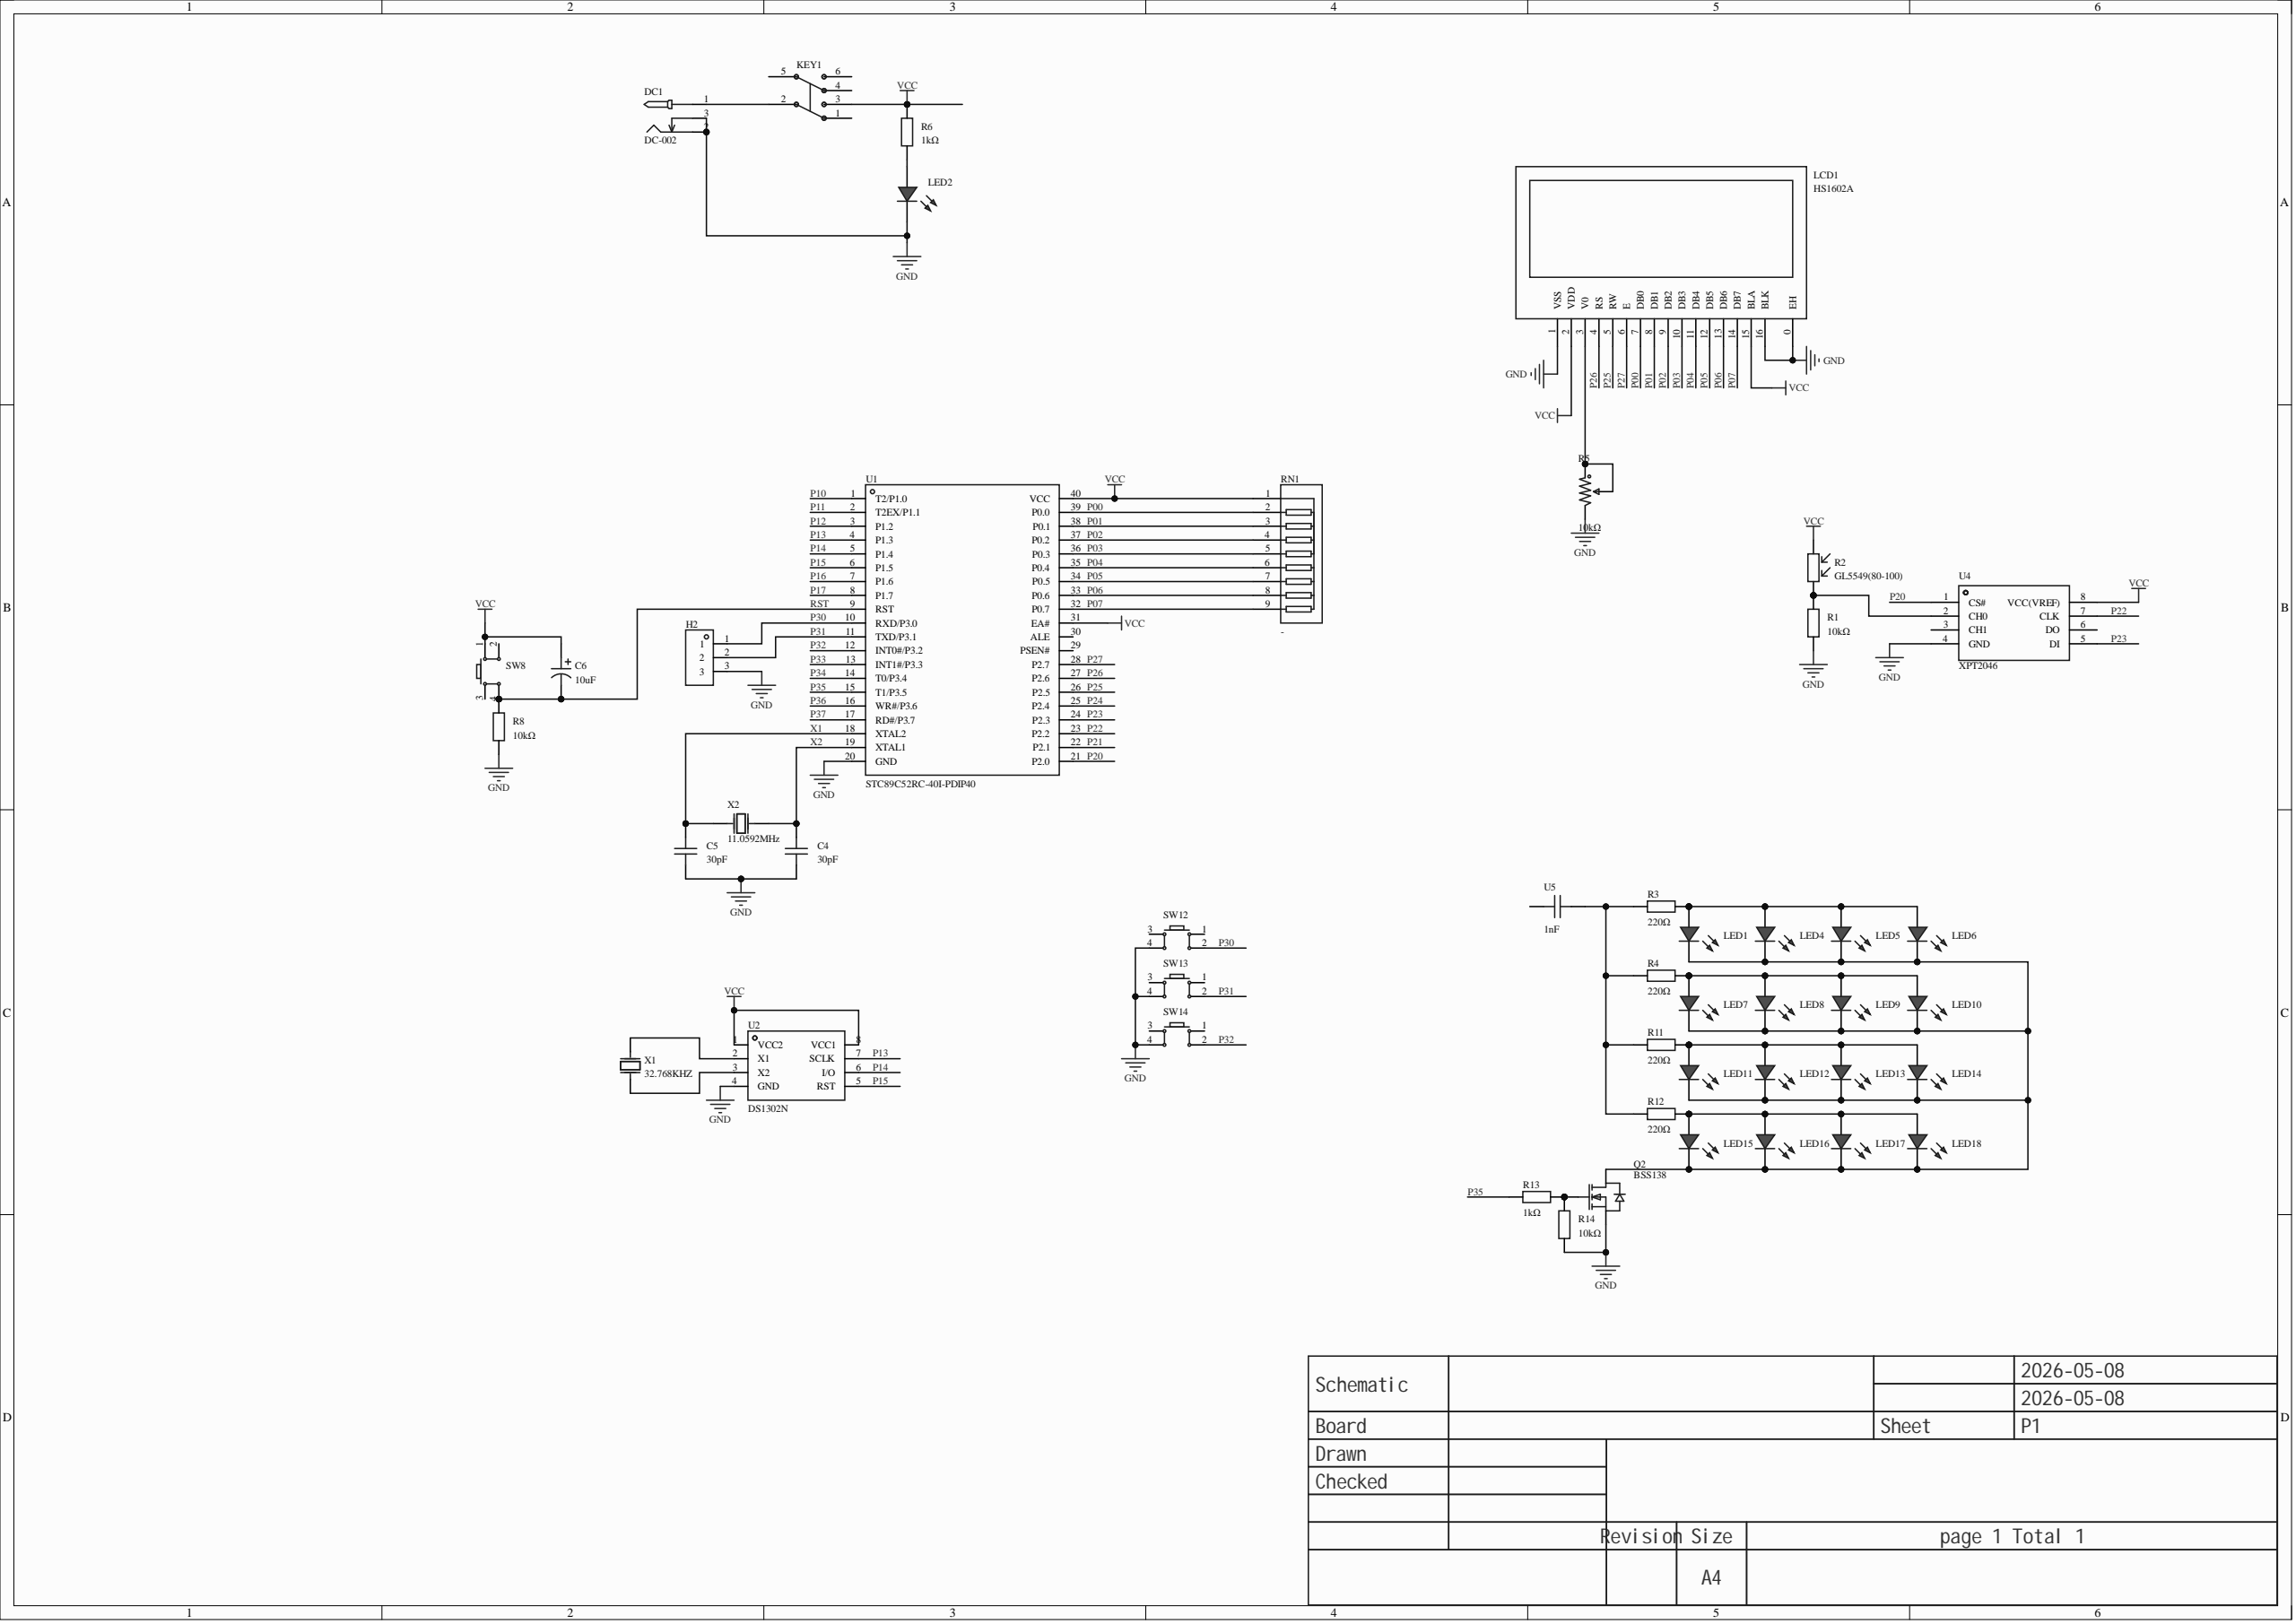Circuit board | Altium Designer | 47 parts | 39 nets
Bill of materials:
Comment,Description,Designator,Footprint,LibRef,Quantity
"30pF","Capacitance: 30pF; tolerance: ±10%; rated voltage: 25V; temperature coefficient: C0G;","C4, C5","CAP-TH_L3.8-W2.5-P2.54-D0.50","C315C300K3G5TA7301","2"
"10uF","Capacitance: 10uF; tolerance: ±20%; rated voltage: 50V; ripple current: 120mA@100KHz; equivalent series resistance (ESR): 1.6Ω;","C6","CAP-TH_BD5.0-P2.00-D0.8-FD-10UF50VC110GL","10UF50VC110GL","1"
"DC-002","","DC1","DC-IN-TH_DC-3510","DC-002","1"
"","","H2","HDR-TH_3P-P2.54-V-M","HDR-M_2.54_1x3P","1"
"Non-latching switch 8.5×8.5 silent","6 pins, 8.5×8.5","KEY1","SW-TH_6P-L8.5-W8.5-P2.54","无自锁开关 8.5×8.5 无声","1"
"HS1602A","Controller: SPLC780; size (inch): 2;","LCD1","LCD1602","HS1602A","1"
"","","LED1, LED2, LED4, LED5, LED6, LED7, LED8, LED9, LED10, LED11, LED12, LED13, LED14, LED15, LED16, LED17, LED18","LED_TH-3mm","LED_TH-R_3mm","17"
"BSS138","","Q2","SOT-23-3_L3.0-W1.7-P0.95-LS2.9-BR","BSS138","1"
"10kΩ","","R1, R8, R14","Res_1/8W","Res_AXIAL-1/8W","3"
"GL5549(80-100)","Dark resistance: 20MΩ; light resistance @10Lux: 80kΩ~150kΩ; spectral peak (wavelength): 540nm;","R2","RES-TH_L5.1-W4.3-P3.40-D0.5","GL5549(80-100)","1"
"220Ω","","R3, R4, R11, R12","Res_1/8W","Res_AXIAL-1/8W","4"
"10kΩ","Resistance: 10kΩ; tolerance: ±25%; power: 100mW;","R5","RES-ADJ-SMD_RM065-V1","RM065-103(10K)","1"
"1kΩ","","R6, R13","Res_1/8W","Res_AXIAL-1/8W","2"
"-","Number of resistors: -; resistance: -; power per element: -;","RN1","RES-ARRAY-TH_9P-P2.54-D1.0","排阻 10 K 5%","1"
"","","SW8, SW12, SW13, SW14","SW-TH_4P-L6.0-W6.0-P4.50-LS6.5","Key_TH_6x6x6","4"
"STC89C52RC-40I-PDIP40","CPU core: 51 family; CPU max frequency: -;","U1","DIP-40_L52.0-W13.7-P2.54-LS15.2-BL","STC89C52RC-40I-PDIP40","1"
"DS1302N","","U2","DIP-8_L9.7-W6.4-P2.54-LS7.6-BL","DS1302N","1"
"XPT2046","","U4","DIP-8_L9.7-W6.4-P2.54-LS7.6-BL","ADC0832CCN","1"
"1nF","","U5","CAP-TH_L5.0-W2.5-P5.00-D1.0","100nF","1"
"32.768KHZ","","X1","HC-49S_L11.5-W5.0-P4.88","8MHZ","1"
"11.059MHz","Crystal type: through-hole crystal; frequency: 11.059MHz; frequency tolerance at room temperature: ±20ppm; load capacitance: 30pF;","X2","OSC-TH_L11.1-W4.7-P4.88","9AC11059302060C3","1"
Netlist (Protel format):
[
C4
CAP-TH_L3.8-W2.5-P2.54-D0.50
30pF



]
[
C5
CAP-TH_L3.8-W2.5-P2.54-D0.50
30pF



]
[
C6
CAP-TH_BD5.0-P2.00-D0.8-FD-10UF50VC110GL
10uF



]
[
DC1
DC-IN-TH_DC-3510
DC-002



]
[
H2
HDR-TH_3P-P2.54-V-M




]
[
KEY1
SW-TH_6P-L8.5-W8.5-P2.54
Non-latching switch 8.5×8.5 silent



]
[
LCD1
LCD1602
HS1602A



]
[
LED1
LED_TH-3mm




]
[
LED2
LED_TH-3mm




]
[
LED4
LED_TH-3mm




]
[
LED5
LED_TH-3mm




]
[
LED6
LED_TH-3mm




]
[
LED7
LED_TH-3mm




]
[
LED8
LED_TH-3mm




]
[
LED9
LED_TH-3mm




]
[
LED10
LED_TH-3mm




]
[
LED11
LED_TH-3mm




]
[
LED12
LED_TH-3mm




]
[
LED13
LED_TH-3mm




]
[
LED14
LED_TH-3mm




]
[
LED15
LED_TH-3mm




]
[
LED16
LED_TH-3mm




]
[
LED17
LED_TH-3mm




]
[
LED18
LED_TH-3mm




]
[
Q2
SOT-23-3_L3.0-W1.7-P0.95-LS2.9-BR
BSS138



]
[
R1
Res_1/8W
10kΩ



]
[
R2
RES-TH_L5.1-W4.3-P3.40-D0.5
GL5549(80-100)



]
[
R3
Res_1/8W
220Ω



]
[
R4
Res_1/8W
220Ω



]
[
R5
RES-ADJ-SMD_RM065-V1
10kΩ



]
[
R6
Res_1/8W
1kΩ



]
[
R8
Res_1/8W
10kΩ



]
[
R11
Res_1/8W
220Ω



]
[
R12
Res_1/8W
220Ω



]
[
R13
Res_1/8W
1kΩ



]
[
R14
Res_1/8W
10kΩ



]
[
RN1
RES-ARRAY-TH_9P-P2.54-D1.0
-



]
[
SW8
SW-TH_4P-L6.0-W6.0-P4.50-LS6.5




]
[
SW12
SW-TH_4P-L6.0-W6.0-P4.50-LS6.5




]
[
SW13
SW-TH_4P-L6.0-W6.0-P4.50-LS6.5




]
[
SW14
SW-TH_4P-L6.0-W6.0-P4.50-LS6.5




]
[
U1
DIP-40_L52.0-W13.7-P2.54-LS15.2-BL
STC89C52RC-40I-PDIP40



]
[
U2
DIP-8_L9.7-W6.4-P2.54-LS7.6-BL
DS1302N



]
[
U4
DIP-8_L9.7-W6.4-P2.54-LS7.6-BL
XPT2046



]
[
U5
CAP-TH_L5.0-W2.5-P5.00-D1.0
1nF



]
[
X1
HC-49S_L11.5-W5.0-P4.88
32.768KHZ



]
[
X2
OSC-TH_L11.1-W4.7-P4.88
11.0592MHz



]
(
X2
C4-2
U1-19
X2-2
)
(
X1
C5-2
U1-18
X2-1
)
(
VCC
C6-1
KEY1-3
LCD1-2
LCD1-15
R2-1
R6-2
RN1-1
SW8-1
U1-31
U1-40
U2-1
U2-8
U4-8
)
(
RST
C6-2
R8-2
SW8-4
U1-9
)
(
P35
R13-1
U1-15
)
(
P32
SW14-2
U1-12
)
(
P31
H2-2
SW13-2
U1-11
)
(
P30
H2-1
SW12-2
U1-10
)
(
P27
LCD1-6
U1-28
)
(
P26
LCD1-4
U1-27
)
(
P25
LCD1-5
U1-26
)
(
P23
U1-24
U4-5
)
(
P22
U1-23
U4-7
)
(
P20
U1-21
U4-1
)
(
P15
U1-6
U2-5
)
(
P14
U1-5
U2-6
)
(
P13
U1-4
U2-7
)
(
P07
LCD1-14
RN1-9
U1-32
)
(
P06
LCD1-13
RN1-8
U1-33
)
(
P05
LCD1-12
RN1-7
U1-34
)
(
P04
LCD1-11
RN1-6
U1-35
)
(
P03
LCD1-10
RN1-5
U1-36
)
(
P02
LCD1-9
RN1-4
U1-37
)
(
P01
LCD1-8
RN1-3
U1-38
)
(
P00
LCD1-7
RN1-2
U1-39
)
(
NetU2_3
U2-3
X1-1
)
(
NetU2_2
U2-2
X1-2
)
(
NetR3_1
R3-1
R4-1
R11-1
R12-1
U5-1
)
(
NetR1_1
R1-1
R2-2
U4-2
)
(
NetQ2_1
Q2-1
R13-2
R14-2
)
(
NetLED15_1
LED15-1
LED16-1
LED17-1
LED18-1
R12-2
)
(
NetLED11_1
LED11-1
LED12-1
LED13-1
LED14-1
R11-2
)
(
NetLED7_1
LED7-1
LED8-1
LED9-1
LED10-1
R4-2
)
(
NetLED2_1
LED2-1
R6-1
)
(
NetLED1_2
LED1-2
LED4-2
LED5-2
LED6-2
LED7-2
LED8-2
LED9-2
LED10-2
LED11-2
LED12-2
LED13-2
LED14-2
LED15-2
LED16-2
LED17-2
LED18-2
Q2-3
)
(
NetLED1_1
LED1-1
LED4-1
LED5-1
LED6-1
R3-2
)
(
NetLCD1_3
LCD1-3
R5-1
R5-2
)
(
NetDC1_1
DC1-1
KEY1-2
)
(
GND
C4-1
C5-1
DC1-2
DC1-3
H2-3
LCD1-0
LCD1-1
LCD1-16
LED2-2
Q2-2
R1-2
R5-3
R8-1
R14-1
SW12-4
SW13-4
SW14-4
U1-20
U2-4
U4-4
)